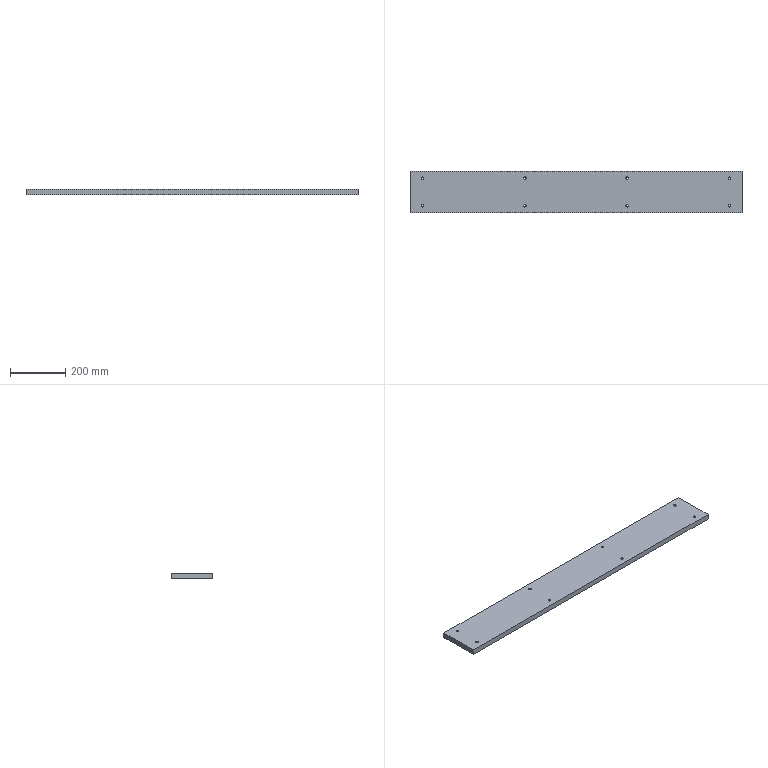Part | SolidWorks | features LPattern 2, Extrusion 1, HoleWzd 1, ICE 1 | 1 solid | 1056 faces | box 1200 x 150 x 20 mm | volume 3476597 mm3 | cylinder 858 | plane 198 | commonest cylinder face diameters 45 x414 39 x412 9 x16 15 x16